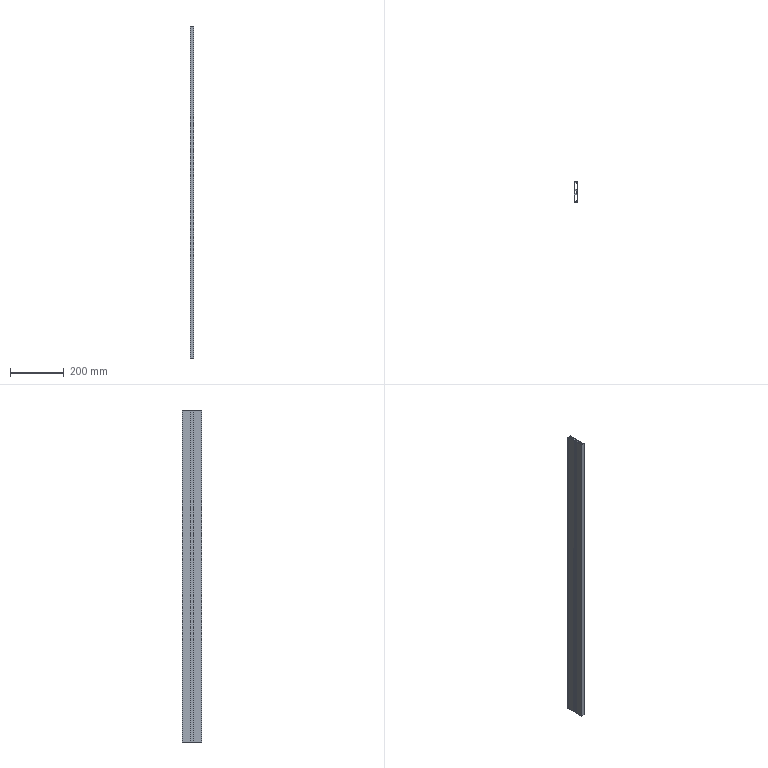Part | 1 solid | 22 faces | box 12 x 73 x 1240 mm | volume 451360 mm3 | plane 22
STEP:
#1=CARTESIAN_POINT('',(-12.,36.5,620.));
#2=VERTEX_POINT('',#1);
#3=CARTESIAN_POINT('',(-12.,4.5,620.));
#4=VERTEX_POINT('',#3);
#5=CARTESIAN_POINT('',(-12.,36.5,620.));
#6=DIRECTION('',(0.,-1.,0.));
#7=VECTOR('',#6,1000.);
#8=LINE('',#5,#7);
#9=EDGE_CURVE('',#2,#4,#8,.T.);
#10=ORIENTED_EDGE('',*,*,#9,.T.);
#11=CARTESIAN_POINT('',(-10.,4.5,620.));
#12=VERTEX_POINT('',#11);
#13=CARTESIAN_POINT('',(-12.,4.5,620.));
#14=DIRECTION('',(1.,0.,0.));
#15=VECTOR('',#14,1000.);
#16=LINE('',#13,#15);
#17=EDGE_CURVE('',#4,#12,#16,.T.);
#18=ORIENTED_EDGE('',*,*,#17,.T.);
#19=CARTESIAN_POINT('',(-10.,6.5,620.));
#20=VERTEX_POINT('',#19);
#21=CARTESIAN_POINT('',(-10.,4.5,620.));
#22=DIRECTION('',(0.,1.,0.));
#23=VECTOR('',#22,1000.);
#24=LINE('',#21,#23);
#25=EDGE_CURVE('',#12,#20,#24,.T.);
#26=ORIENTED_EDGE('',*,*,#25,.T.);
#27=CARTESIAN_POINT('',(-4.,6.5,620.));
#28=VERTEX_POINT('',#27);
#29=CARTESIAN_POINT('',(-10.,6.5,620.));
#30=DIRECTION('',(1.,0.,0.));
#31=VECTOR('',#30,1000.);
#32=LINE('',#29,#31);
#33=EDGE_CURVE('',#20,#28,#32,.T.);
#34=ORIENTED_EDGE('',*,*,#33,.T.);
#35=CARTESIAN_POINT('',(-4.,-6.5,620.));
#36=VERTEX_POINT('',#35);
#37=CARTESIAN_POINT('',(-4.,6.5,620.));
#38=DIRECTION('',(0.,-1.,0.));
#39=VECTOR('',#38,1000.);
#40=LINE('',#37,#39);
#41=EDGE_CURVE('',#28,#36,#40,.T.);
#42=ORIENTED_EDGE('',*,*,#41,.T.);
#43=CARTESIAN_POINT('',(-10.,-6.5,620.));
#44=VERTEX_POINT('',#43);
#45=CARTESIAN_POINT('',(-4.,-6.5,620.));
#46=DIRECTION('',(-1.,0.,0.));
#47=VECTOR('',#46,1000.);
#48=LINE('',#45,#47);
#49=EDGE_CURVE('',#36,#44,#48,.T.);
#50=ORIENTED_EDGE('',*,*,#49,.T.);
#51=CARTESIAN_POINT('',(-10.,-4.5,620.));
#52=VERTEX_POINT('',#51);
#53=CARTESIAN_POINT('',(-10.,-6.5,620.));
#54=DIRECTION('',(0.,1.,0.));
#55=VECTOR('',#54,1000.);
#56=LINE('',#53,#55);
#57=EDGE_CURVE('',#44,#52,#56,.T.);
#58=ORIENTED_EDGE('',*,*,#57,.T.);
#59=CARTESIAN_POINT('',(-12.,-4.5,620.));
#60=VERTEX_POINT('',#59);
#61=CARTESIAN_POINT('',(-10.,-4.5,620.));
#62=DIRECTION('',(-1.,0.,0.));
#63=VECTOR('',#62,1000.);
#64=LINE('',#61,#63);
#65=EDGE_CURVE('',#52,#60,#64,.T.);
#66=ORIENTED_EDGE('',*,*,#65,.T.);
#67=CARTESIAN_POINT('',(-12.,-36.5,620.));
#68=VERTEX_POINT('',#67);
#69=CARTESIAN_POINT('',(-12.,-4.5,620.));
#70=DIRECTION('',(0.,-1.,0.));
#71=VECTOR('',#70,1000.);
#72=LINE('',#69,#71);
#73=EDGE_CURVE('',#60,#68,#72,.T.);
#74=ORIENTED_EDGE('',*,*,#73,.T.);
#75=CARTESIAN_POINT('',(0.,-36.5,620.));
#76=VERTEX_POINT('',#75);
#77=CARTESIAN_POINT('',(-12.,-36.5,620.));
#78=DIRECTION('',(1.,0.,0.));
#79=VECTOR('',#78,1000.);
#80=LINE('',#77,#79);
#81=EDGE_CURVE('',#68,#76,#80,.T.);
#82=ORIENTED_EDGE('',*,*,#81,.T.);
#83=CARTESIAN_POINT('',(0.,36.5,620.));
#84=VERTEX_POINT('',#83);
#85=CARTESIAN_POINT('',(0.,-36.5,620.));
#86=DIRECTION('',(0.,1.,0.));
#87=VECTOR('',#86,1000.);
#88=LINE('',#85,#87);
#89=EDGE_CURVE('',#76,#84,#88,.T.);
#90=ORIENTED_EDGE('',*,*,#89,.T.);
#91=CARTESIAN_POINT('',(0.,36.5,620.));
#92=DIRECTION('',(-1.,0.,0.));
#93=VECTOR('',#92,1000.);
#94=LINE('',#91,#93);
#95=EDGE_CURVE('',#84,#2,#94,.T.);
#96=ORIENTED_EDGE('',*,*,#95,.T.);
#97=EDGE_LOOP('',(#10,#18,#26,#34,#42,#50,#58,#66,#74,#82,#90,#96));
#98=FACE_OUTER_BOUND('',#97,.T.);
#99=CARTESIAN_POINT('',(-10.,-34.5,620.));
#100=VERTEX_POINT('',#99);
#101=CARTESIAN_POINT('',(-2.,-34.5,620.));
#102=VERTEX_POINT('',#101);
#103=CARTESIAN_POINT('',(-2.,-34.5,620.));
#104=DIRECTION('',(1.,0.,0.));
#105=VECTOR('',#104,1000.);
#106=LINE('',#103,#105);
#107=EDGE_CURVE('',#100,#102,#106,.T.);
#108=ORIENTED_EDGE('',*,*,#107,.F.);
#109=CARTESIAN_POINT('',(-10.,-8.5,620.));
#110=VERTEX_POINT('',#109);
#111=CARTESIAN_POINT('',(-10.,-34.5,620.));
#112=DIRECTION('',(0.,-1.,0.));
#113=VECTOR('',#112,1000.);
#114=LINE('',#111,#113);
#115=EDGE_CURVE('',#110,#100,#114,.T.);
#116=ORIENTED_EDGE('',*,*,#115,.F.);
#117=CARTESIAN_POINT('',(-2.,-8.5,620.));
#118=VERTEX_POINT('',#117);
#119=CARTESIAN_POINT('',(-10.,-8.5,620.));
#120=DIRECTION('',(-1.,0.,0.));
#121=VECTOR('',#120,1000.);
#122=LINE('',#119,#121);
#123=EDGE_CURVE('',#118,#110,#122,.T.);
#124=ORIENTED_EDGE('',*,*,#123,.F.);
#125=CARTESIAN_POINT('',(-2.,-8.5,620.));
#126=DIRECTION('',(0.,1.,0.));
#127=VECTOR('',#126,1000.);
#128=LINE('',#125,#127);
#129=EDGE_CURVE('',#102,#118,#128,.T.);
#130=ORIENTED_EDGE('',*,*,#129,.F.);
#131=EDGE_LOOP('',(#108,#116,#124,#130));
#132=FACE_BOUND('',#131,.T.);
#133=CARTESIAN_POINT('',(-10.,34.5,620.));
#134=VERTEX_POINT('',#133);
#135=CARTESIAN_POINT('',(-10.,8.5,620.));
#136=VERTEX_POINT('',#135);
#137=CARTESIAN_POINT('',(-10.,8.5,620.));
#138=DIRECTION('',(0.,-1.,0.));
#139=VECTOR('',#138,1000.);
#140=LINE('',#137,#139);
#141=EDGE_CURVE('',#134,#136,#140,.T.);
#142=ORIENTED_EDGE('',*,*,#141,.F.);
#143=CARTESIAN_POINT('',(-2.,34.5,620.));
#144=VERTEX_POINT('',#143);
#145=CARTESIAN_POINT('',(-10.,34.5,620.));
#146=DIRECTION('',(-1.,0.,0.));
#147=VECTOR('',#146,1000.);
#148=LINE('',#145,#147);
#149=EDGE_CURVE('',#144,#134,#148,.T.);
#150=ORIENTED_EDGE('',*,*,#149,.F.);
#151=CARTESIAN_POINT('',(-2.,8.5,620.));
#152=VERTEX_POINT('',#151);
#153=CARTESIAN_POINT('',(-2.,34.5,620.));
#154=DIRECTION('',(0.,1.,0.));
#155=VECTOR('',#154,1000.);
#156=LINE('',#153,#155);
#157=EDGE_CURVE('',#152,#144,#156,.T.);
#158=ORIENTED_EDGE('',*,*,#157,.F.);
#159=CARTESIAN_POINT('',(-2.,8.5,620.));
#160=DIRECTION('',(1.,0.,0.));
#161=VECTOR('',#160,1000.);
#162=LINE('',#159,#161);
#163=EDGE_CURVE('',#136,#152,#162,.T.);
#164=ORIENTED_EDGE('',*,*,#163,.F.);
#165=EDGE_LOOP('',(#142,#150,#158,#164));
#166=FACE_BOUND('',#165,.T.);
#167=CARTESIAN_POINT('',(0.,0.,620.));
#168=DIRECTION('',(0.,0.,1.));
#169=DIRECTION('',(1.,0.,0.));
#170=AXIS2_PLACEMENT_3D('',#167,#168,#169);
#171=PLANE('',#170);
#172=ADVANCED_FACE('',(#98,#132,#166),#171,.T.);
#173=CARTESIAN_POINT('',(-10.,-8.5,-620.));
#174=VERTEX_POINT('',#173);
#175=CARTESIAN_POINT('',(-10.,-34.5,-620.));
#176=VERTEX_POINT('',#175);
#177=CARTESIAN_POINT('',(-10.,-34.5,-620.));
#178=DIRECTION('',(0.,-1.,0.));
#179=VECTOR('',#178,1000.);
#180=LINE('',#177,#179);
#181=EDGE_CURVE('',#174,#176,#180,.T.);
#182=ORIENTED_EDGE('',*,*,#181,.T.);
#183=CARTESIAN_POINT('',(-2.,-34.5,-620.));
#184=VERTEX_POINT('',#183);
#185=CARTESIAN_POINT('',(-2.,-34.5,-620.));
#186=DIRECTION('',(1.,0.,0.));
#187=VECTOR('',#186,1000.);
#188=LINE('',#185,#187);
#189=EDGE_CURVE('',#176,#184,#188,.T.);
#190=ORIENTED_EDGE('',*,*,#189,.T.);
#191=CARTESIAN_POINT('',(-2.,-8.5,-620.));
#192=VERTEX_POINT('',#191);
#193=CARTESIAN_POINT('',(-2.,-8.5,-620.));
#194=DIRECTION('',(0.,1.,0.));
#195=VECTOR('',#194,1000.);
#196=LINE('',#193,#195);
#197=EDGE_CURVE('',#184,#192,#196,.T.);
#198=ORIENTED_EDGE('',*,*,#197,.T.);
#199=CARTESIAN_POINT('',(-10.,-8.5,-620.));
#200=DIRECTION('',(-1.,0.,0.));
#201=VECTOR('',#200,1000.);
#202=LINE('',#199,#201);
#203=EDGE_CURVE('',#192,#174,#202,.T.);
#204=ORIENTED_EDGE('',*,*,#203,.T.);
#205=EDGE_LOOP('',(#182,#190,#198,#204));
#206=FACE_BOUND('',#205,.T.);
#207=CARTESIAN_POINT('',(-12.,36.5,-620.));
#208=VERTEX_POINT('',#207);
#209=CARTESIAN_POINT('',(-12.,4.5,-620.));
#210=VERTEX_POINT('',#209);
#211=CARTESIAN_POINT('',(-12.,36.5,-620.));
#212=DIRECTION('',(0.,-1.,0.));
#213=VECTOR('',#212,1000.);
#214=LINE('',#211,#213);
#215=EDGE_CURVE('',#208,#210,#214,.T.);
#216=ORIENTED_EDGE('',*,*,#215,.F.);
#217=CARTESIAN_POINT('',(0.,36.5,-620.));
#218=VERTEX_POINT('',#217);
#219=CARTESIAN_POINT('',(0.,36.5,-620.));
#220=DIRECTION('',(-1.,0.,0.));
#221=VECTOR('',#220,1000.);
#222=LINE('',#219,#221);
#223=EDGE_CURVE('',#218,#208,#222,.T.);
#224=ORIENTED_EDGE('',*,*,#223,.F.);
#225=CARTESIAN_POINT('',(0.,-36.5,-620.));
#226=VERTEX_POINT('',#225);
#227=CARTESIAN_POINT('',(0.,-36.5,-620.));
#228=DIRECTION('',(0.,1.,0.));
#229=VECTOR('',#228,1000.);
#230=LINE('',#227,#229);
#231=EDGE_CURVE('',#226,#218,#230,.T.);
#232=ORIENTED_EDGE('',*,*,#231,.F.);
#233=CARTESIAN_POINT('',(-12.,-36.5,-620.));
#234=VERTEX_POINT('',#233);
#235=CARTESIAN_POINT('',(-12.,-36.5,-620.));
#236=DIRECTION('',(1.,0.,0.));
#237=VECTOR('',#236,1000.);
#238=LINE('',#235,#237);
#239=EDGE_CURVE('',#234,#226,#238,.T.);
#240=ORIENTED_EDGE('',*,*,#239,.F.);
#241=CARTESIAN_POINT('',(-12.,-4.5,-620.));
#242=VERTEX_POINT('',#241);
#243=CARTESIAN_POINT('',(-12.,-4.5,-620.));
#244=DIRECTION('',(0.,-1.,0.));
#245=VECTOR('',#244,1000.);
#246=LINE('',#243,#245);
#247=EDGE_CURVE('',#242,#234,#246,.T.);
#248=ORIENTED_EDGE('',*,*,#247,.F.);
#249=CARTESIAN_POINT('',(-10.,-4.5,-620.));
#250=VERTEX_POINT('',#249);
#251=CARTESIAN_POINT('',(-10.,-4.5,-620.));
#252=DIRECTION('',(-1.,0.,0.));
#253=VECTOR('',#252,1000.);
#254=LINE('',#251,#253);
#255=EDGE_CURVE('',#250,#242,#254,.T.);
#256=ORIENTED_EDGE('',*,*,#255,.F.);
#257=CARTESIAN_POINT('',(-10.,-6.5,-620.));
#258=VERTEX_POINT('',#257);
#259=CARTESIAN_POINT('',(-10.,-6.5,-620.));
#260=DIRECTION('',(0.,1.,0.));
#261=VECTOR('',#260,1000.);
#262=LINE('',#259,#261);
#263=EDGE_CURVE('',#258,#250,#262,.T.);
#264=ORIENTED_EDGE('',*,*,#263,.F.);
#265=CARTESIAN_POINT('',(-4.,-6.5,-620.));
#266=VERTEX_POINT('',#265);
#267=CARTESIAN_POINT('',(-4.,-6.5,-620.));
#268=DIRECTION('',(-1.,0.,0.));
#269=VECTOR('',#268,1000.);
#270=LINE('',#267,#269);
#271=EDGE_CURVE('',#266,#258,#270,.T.);
#272=ORIENTED_EDGE('',*,*,#271,.F.);
#273=CARTESIAN_POINT('',(-4.,6.5,-620.));
#274=VERTEX_POINT('',#273);
#275=CARTESIAN_POINT('',(-4.,6.5,-620.));
#276=DIRECTION('',(0.,-1.,0.));
#277=VECTOR('',#276,1000.);
#278=LINE('',#275,#277);
#279=EDGE_CURVE('',#274,#266,#278,.T.);
#280=ORIENTED_EDGE('',*,*,#279,.F.);
#281=CARTESIAN_POINT('',(-10.,6.5,-620.));
#282=VERTEX_POINT('',#281);
#283=CARTESIAN_POINT('',(-10.,6.5,-620.));
#284=DIRECTION('',(1.,0.,0.));
#285=VECTOR('',#284,1000.);
#286=LINE('',#283,#285);
#287=EDGE_CURVE('',#282,#274,#286,.T.);
#288=ORIENTED_EDGE('',*,*,#287,.F.);
#289=CARTESIAN_POINT('',(-10.,4.5,-620.));
#290=VERTEX_POINT('',#289);
#291=CARTESIAN_POINT('',(-10.,4.5,-620.));
#292=DIRECTION('',(0.,1.,0.));
#293=VECTOR('',#292,1000.);
#294=LINE('',#291,#293);
#295=EDGE_CURVE('',#290,#282,#294,.T.);
#296=ORIENTED_EDGE('',*,*,#295,.F.);
#297=CARTESIAN_POINT('',(-12.,4.5,-620.));
#298=DIRECTION('',(1.,0.,0.));
#299=VECTOR('',#298,1000.);
#300=LINE('',#297,#299);
#301=EDGE_CURVE('',#210,#290,#300,.T.);
#302=ORIENTED_EDGE('',*,*,#301,.F.);
#303=EDGE_LOOP('',(#216,#224,#232,#240,#248,#256,#264,#272,#280,#288,#296,#302));
#304=FACE_OUTER_BOUND('',#303,.T.);
#305=CARTESIAN_POINT('',(-2.,34.5,-620.));
#306=VERTEX_POINT('',#305);
#307=CARTESIAN_POINT('',(-10.,34.5,-620.));
#308=VERTEX_POINT('',#307);
#309=CARTESIAN_POINT('',(-10.,34.5,-620.));
#310=DIRECTION('',(-1.,0.,0.));
#311=VECTOR('',#310,1000.);
#312=LINE('',#309,#311);
#313=EDGE_CURVE('',#306,#308,#312,.T.);
#314=ORIENTED_EDGE('',*,*,#313,.T.);
#315=CARTESIAN_POINT('',(-10.,8.5,-620.));
#316=VERTEX_POINT('',#315);
#317=CARTESIAN_POINT('',(-10.,8.5,-620.));
#318=DIRECTION('',(0.,-1.,0.));
#319=VECTOR('',#318,1000.);
#320=LINE('',#317,#319);
#321=EDGE_CURVE('',#308,#316,#320,.T.);
#322=ORIENTED_EDGE('',*,*,#321,.T.);
#323=CARTESIAN_POINT('',(-2.,8.5,-620.));
#324=VERTEX_POINT('',#323);
#325=CARTESIAN_POINT('',(-2.,8.5,-620.));
#326=DIRECTION('',(1.,0.,0.));
#327=VECTOR('',#326,1000.);
#328=LINE('',#325,#327);
#329=EDGE_CURVE('',#316,#324,#328,.T.);
#330=ORIENTED_EDGE('',*,*,#329,.T.);
#331=CARTESIAN_POINT('',(-2.,34.5,-620.));
#332=DIRECTION('',(0.,1.,0.));
#333=VECTOR('',#332,1000.);
#334=LINE('',#331,#333);
#335=EDGE_CURVE('',#324,#306,#334,.T.);
#336=ORIENTED_EDGE('',*,*,#335,.T.);
#337=EDGE_LOOP('',(#314,#322,#330,#336));
#338=FACE_BOUND('',#337,.T.);
#339=CARTESIAN_POINT('',(0.,0.,-620.));
#340=DIRECTION('',(0.,0.,1.));
#341=DIRECTION('',(1.,0.,0.));
#342=AXIS2_PLACEMENT_3D('',#339,#340,#341);
#343=PLANE('',#342);
#344=ADVANCED_FACE('',(#206,#304,#338),#343,.F.);
#345=ORIENTED_EDGE('',*,*,#215,.T.);
#346=CARTESIAN_POINT('',(-12.,4.5,620.));
#347=DIRECTION('',(0.,0.,-1.));
#348=VECTOR('',#347,1000.);
#349=LINE('',#346,#348);
#350=EDGE_CURVE('',#4,#210,#349,.T.);
#351=ORIENTED_EDGE('',*,*,#350,.F.);
#352=ORIENTED_EDGE('',*,*,#9,.F.);
#353=CARTESIAN_POINT('',(-12.,36.5,620.));
#354=DIRECTION('',(0.,0.,-1.));
#355=VECTOR('',#354,1000.);
#356=LINE('',#353,#355);
#357=EDGE_CURVE('',#2,#208,#356,.T.);
#358=ORIENTED_EDGE('',*,*,#357,.T.);
#359=EDGE_LOOP('',(#345,#351,#352,#358));
#360=FACE_OUTER_BOUND('',#359,.T.);
#361=CARTESIAN_POINT('',(-12.,36.5,620.));
#362=DIRECTION('',(1.,0.,0.));
#363=DIRECTION('',(0.,0.,-1.));
#364=AXIS2_PLACEMENT_3D('',#361,#362,#363);
#365=PLANE('',#364);
#366=ADVANCED_FACE('',(#360),#365,.F.);
#367=ORIENTED_EDGE('',*,*,#301,.T.);
#368=CARTESIAN_POINT('',(-10.,4.5,620.));
#369=DIRECTION('',(0.,0.,-1.));
#370=VECTOR('',#369,1000.);
#371=LINE('',#368,#370);
#372=EDGE_CURVE('',#12,#290,#371,.T.);
#373=ORIENTED_EDGE('',*,*,#372,.F.);
#374=ORIENTED_EDGE('',*,*,#17,.F.);
#375=ORIENTED_EDGE('',*,*,#350,.T.);
#376=EDGE_LOOP('',(#367,#373,#374,#375));
#377=FACE_OUTER_BOUND('',#376,.T.);
#378=CARTESIAN_POINT('',(-12.,4.5,620.));
#379=DIRECTION('',(0.,1.,0.));
#380=DIRECTION('',(0.,0.,1.));
#381=AXIS2_PLACEMENT_3D('',#378,#379,#380);
#382=PLANE('',#381);
#383=ADVANCED_FACE('',(#377),#382,.F.);
#384=ORIENTED_EDGE('',*,*,#295,.T.);
#385=CARTESIAN_POINT('',(-10.,6.5,620.));
#386=DIRECTION('',(0.,0.,-1.));
#387=VECTOR('',#386,1000.);
#388=LINE('',#385,#387);
#389=EDGE_CURVE('',#20,#282,#388,.T.);
#390=ORIENTED_EDGE('',*,*,#389,.F.);
#391=ORIENTED_EDGE('',*,*,#25,.F.);
#392=ORIENTED_EDGE('',*,*,#372,.T.);
#393=EDGE_LOOP('',(#384,#390,#391,#392));
#394=FACE_OUTER_BOUND('',#393,.T.);
#395=CARTESIAN_POINT('',(-10.,4.5,620.));
#396=DIRECTION('',(-1.,0.,0.));
#397=DIRECTION('',(0.,0.,1.));
#398=AXIS2_PLACEMENT_3D('',#395,#396,#397);
#399=PLANE('',#398);
#400=ADVANCED_FACE('',(#394),#399,.F.);
#401=ORIENTED_EDGE('',*,*,#287,.T.);
#402=CARTESIAN_POINT('',(-4.,6.5,620.));
#403=DIRECTION('',(0.,0.,-1.));
#404=VECTOR('',#403,1000.);
#405=LINE('',#402,#404);
#406=EDGE_CURVE('',#28,#274,#405,.T.);
#407=ORIENTED_EDGE('',*,*,#406,.F.);
#408=ORIENTED_EDGE('',*,*,#33,.F.);
#409=ORIENTED_EDGE('',*,*,#389,.T.);
#410=EDGE_LOOP('',(#401,#407,#408,#409));
#411=FACE_OUTER_BOUND('',#410,.T.);
#412=CARTESIAN_POINT('',(-10.,6.5,620.));
#413=DIRECTION('',(0.,1.,0.));
#414=DIRECTION('',(0.,0.,1.));
#415=AXIS2_PLACEMENT_3D('',#412,#413,#414);
#416=PLANE('',#415);
#417=ADVANCED_FACE('',(#411),#416,.F.);
#418=ORIENTED_EDGE('',*,*,#279,.T.);
#419=CARTESIAN_POINT('',(-4.,-6.5,620.));
#420=DIRECTION('',(0.,0.,-1.));
#421=VECTOR('',#420,1000.);
#422=LINE('',#419,#421);
#423=EDGE_CURVE('',#36,#266,#422,.T.);
#424=ORIENTED_EDGE('',*,*,#423,.F.);
#425=ORIENTED_EDGE('',*,*,#41,.F.);
#426=ORIENTED_EDGE('',*,*,#406,.T.);
#427=EDGE_LOOP('',(#418,#424,#425,#426));
#428=FACE_OUTER_BOUND('',#427,.T.);
#429=CARTESIAN_POINT('',(-4.,6.5,620.));
#430=DIRECTION('',(1.,0.,0.));
#431=DIRECTION('',(0.,0.,-1.));
#432=AXIS2_PLACEMENT_3D('',#429,#430,#431);
#433=PLANE('',#432);
#434=ADVANCED_FACE('',(#428),#433,.F.);
#435=ORIENTED_EDGE('',*,*,#271,.T.);
#436=CARTESIAN_POINT('',(-10.,-6.5,620.));
#437=DIRECTION('',(0.,0.,-1.));
#438=VECTOR('',#437,1000.);
#439=LINE('',#436,#438);
#440=EDGE_CURVE('',#44,#258,#439,.T.);
#441=ORIENTED_EDGE('',*,*,#440,.F.);
#442=ORIENTED_EDGE('',*,*,#49,.F.);
#443=ORIENTED_EDGE('',*,*,#423,.T.);
#444=EDGE_LOOP('',(#435,#441,#442,#443));
#445=FACE_OUTER_BOUND('',#444,.T.);
#446=CARTESIAN_POINT('',(-4.,-6.5,620.));
#447=DIRECTION('',(0.,-1.,0.));
#448=DIRECTION('',(0.,0.,-1.));
#449=AXIS2_PLACEMENT_3D('',#446,#447,#448);
#450=PLANE('',#449);
#451=ADVANCED_FACE('',(#445),#450,.F.);
#452=ORIENTED_EDGE('',*,*,#263,.T.);
#453=CARTESIAN_POINT('',(-10.,-4.5,620.));
#454=DIRECTION('',(0.,0.,-1.));
#455=VECTOR('',#454,1000.);
#456=LINE('',#453,#455);
#457=EDGE_CURVE('',#52,#250,#456,.T.);
#458=ORIENTED_EDGE('',*,*,#457,.F.);
#459=ORIENTED_EDGE('',*,*,#57,.F.);
#460=ORIENTED_EDGE('',*,*,#440,.T.);
#461=EDGE_LOOP('',(#452,#458,#459,#460));
#462=FACE_OUTER_BOUND('',#461,.T.);
#463=CARTESIAN_POINT('',(-10.,-6.5,620.));
#464=DIRECTION('',(-1.,0.,0.));
#465=DIRECTION('',(0.,0.,1.));
#466=AXIS2_PLACEMENT_3D('',#463,#464,#465);
#467=PLANE('',#466);
#468=ADVANCED_FACE('',(#462),#467,.F.);
#469=ORIENTED_EDGE('',*,*,#255,.T.);
#470=CARTESIAN_POINT('',(-12.,-4.5,620.));
#471=DIRECTION('',(0.,0.,-1.));
#472=VECTOR('',#471,1000.);
#473=LINE('',#470,#472);
#474=EDGE_CURVE('',#60,#242,#473,.T.);
#475=ORIENTED_EDGE('',*,*,#474,.F.);
#476=ORIENTED_EDGE('',*,*,#65,.F.);
#477=ORIENTED_EDGE('',*,*,#457,.T.);
#478=EDGE_LOOP('',(#469,#475,#476,#477));
#479=FACE_OUTER_BOUND('',#478,.T.);
#480=CARTESIAN_POINT('',(-10.,-4.5,620.));
#481=DIRECTION('',(0.,-1.,0.));
#482=DIRECTION('',(0.,0.,-1.));
#483=AXIS2_PLACEMENT_3D('',#480,#481,#482);
#484=PLANE('',#483);
#485=ADVANCED_FACE('',(#479),#484,.F.);
#486=ORIENTED_EDGE('',*,*,#247,.T.);
#487=CARTESIAN_POINT('',(-12.,-36.5,620.));
#488=DIRECTION('',(0.,0.,-1.));
#489=VECTOR('',#488,1000.);
#490=LINE('',#487,#489);
#491=EDGE_CURVE('',#68,#234,#490,.T.);
#492=ORIENTED_EDGE('',*,*,#491,.F.);
#493=ORIENTED_EDGE('',*,*,#73,.F.);
#494=ORIENTED_EDGE('',*,*,#474,.T.);
#495=EDGE_LOOP('',(#486,#492,#493,#494));
#496=FACE_OUTER_BOUND('',#495,.T.);
#497=CARTESIAN_POINT('',(-12.,-4.5,620.));
#498=DIRECTION('',(1.,0.,0.));
#499=DIRECTION('',(0.,0.,-1.));
#500=AXIS2_PLACEMENT_3D('',#497,#498,#499);
#501=PLANE('',#500);
#502=ADVANCED_FACE('',(#496),#501,.F.);
#503=ORIENTED_EDGE('',*,*,#239,.T.);
#504=CARTESIAN_POINT('',(0.,-36.5,620.));
#505=DIRECTION('',(0.,0.,-1.));
#506=VECTOR('',#505,1000.);
#507=LINE('',#504,#506);
#508=EDGE_CURVE('',#76,#226,#507,.T.);
#509=ORIENTED_EDGE('',*,*,#508,.F.);
#510=ORIENTED_EDGE('',*,*,#81,.F.);
#511=ORIENTED_EDGE('',*,*,#491,.T.);
#512=EDGE_LOOP('',(#503,#509,#510,#511));
#513=FACE_OUTER_BOUND('',#512,.T.);
#514=CARTESIAN_POINT('',(-12.,-36.5,620.));
#515=DIRECTION('',(0.,1.,0.));
#516=DIRECTION('',(0.,0.,1.));
#517=AXIS2_PLACEMENT_3D('',#514,#515,#516);
#518=PLANE('',#517);
#519=ADVANCED_FACE('',(#513),#518,.F.);
#520=ORIENTED_EDGE('',*,*,#231,.T.);
#521=CARTESIAN_POINT('',(0.,36.5,620.));
#522=DIRECTION('',(0.,0.,-1.));
#523=VECTOR('',#522,1000.);
#524=LINE('',#521,#523);
#525=EDGE_CURVE('',#84,#218,#524,.T.);
#526=ORIENTED_EDGE('',*,*,#525,.F.);
#527=ORIENTED_EDGE('',*,*,#89,.F.);
#528=ORIENTED_EDGE('',*,*,#508,.T.);
#529=EDGE_LOOP('',(#520,#526,#527,#528));
#530=FACE_OUTER_BOUND('',#529,.T.);
#531=CARTESIAN_POINT('',(0.,-36.5,620.));
#532=DIRECTION('',(-1.,0.,0.));
#533=DIRECTION('',(0.,0.,1.));
#534=AXIS2_PLACEMENT_3D('',#531,#532,#533);
#535=PLANE('',#534);
#536=ADVANCED_FACE('',(#530),#535,.F.);
#537=ORIENTED_EDGE('',*,*,#223,.T.);
#538=ORIENTED_EDGE('',*,*,#357,.F.);
#539=ORIENTED_EDGE('',*,*,#95,.F.);
#540=ORIENTED_EDGE('',*,*,#525,.T.);
#541=EDGE_LOOP('',(#537,#538,#539,#540));
#542=FACE_OUTER_BOUND('',#541,.T.);
#543=CARTESIAN_POINT('',(0.,36.5,620.));
#544=DIRECTION('',(0.,-1.,0.));
#545=DIRECTION('',(0.,0.,-1.));
#546=AXIS2_PLACEMENT_3D('',#543,#544,#545);
#547=PLANE('',#546);
#548=ADVANCED_FACE('',(#542),#547,.F.);
#549=ORIENTED_EDGE('',*,*,#181,.F.);
#550=CARTESIAN_POINT('',(-10.,-8.5,620.));
#551=DIRECTION('',(0.,0.,-1.));
#552=VECTOR('',#551,1000.);
#553=LINE('',#550,#552);
#554=EDGE_CURVE('',#110,#174,#553,.T.);
#555=ORIENTED_EDGE('',*,*,#554,.F.);
#556=ORIENTED_EDGE('',*,*,#115,.T.);
#557=CARTESIAN_POINT('',(-10.,-34.5,620.));
#558=DIRECTION('',(0.,0.,-1.));
#559=VECTOR('',#558,1000.);
#560=LINE('',#557,#559);
#561=EDGE_CURVE('',#100,#176,#560,.T.);
#562=ORIENTED_EDGE('',*,*,#561,.T.);
#563=EDGE_LOOP('',(#549,#555,#556,#562));
#564=FACE_OUTER_BOUND('',#563,.T.);
#565=CARTESIAN_POINT('',(-10.,-34.5,620.));
#566=DIRECTION('',(1.,0.,0.));
#567=DIRECTION('',(0.,0.,-1.));
#568=AXIS2_PLACEMENT_3D('',#565,#566,#567);
#569=PLANE('',#568);
#570=ADVANCED_FACE('',(#564),#569,.T.);
#571=ORIENTED_EDGE('',*,*,#189,.F.);
#572=ORIENTED_EDGE('',*,*,#561,.F.);
#573=ORIENTED_EDGE('',*,*,#107,.T.);
#574=CARTESIAN_POINT('',(-2.,-34.5,620.));
#575=DIRECTION('',(0.,0.,-1.));
#576=VECTOR('',#575,1000.);
#577=LINE('',#574,#576);
#578=EDGE_CURVE('',#102,#184,#577,.T.);
#579=ORIENTED_EDGE('',*,*,#578,.T.);
#580=EDGE_LOOP('',(#571,#572,#573,#579));
#581=FACE_OUTER_BOUND('',#580,.T.);
#582=CARTESIAN_POINT('',(-2.,-34.5,620.));
#583=DIRECTION('',(0.,1.,0.));
#584=DIRECTION('',(0.,0.,1.));
#585=AXIS2_PLACEMENT_3D('',#582,#583,#584);
#586=PLANE('',#585);
#587=ADVANCED_FACE('',(#581),#586,.T.);
#588=ORIENTED_EDGE('',*,*,#197,.F.);
#589=ORIENTED_EDGE('',*,*,#578,.F.);
#590=ORIENTED_EDGE('',*,*,#129,.T.);
#591=CARTESIAN_POINT('',(-2.,-8.5,620.));
#592=DIRECTION('',(0.,0.,-1.));
#593=VECTOR('',#592,1000.);
#594=LINE('',#591,#593);
#595=EDGE_CURVE('',#118,#192,#594,.T.);
#596=ORIENTED_EDGE('',*,*,#595,.T.);
#597=EDGE_LOOP('',(#588,#589,#590,#596));
#598=FACE_OUTER_BOUND('',#597,.T.);
#599=CARTESIAN_POINT('',(-2.,-8.5,620.));
#600=DIRECTION('',(-1.,0.,0.));
#601=DIRECTION('',(0.,0.,1.));
#602=AXIS2_PLACEMENT_3D('',#599,#600,#601);
#603=PLANE('',#602);
#604=ADVANCED_FACE('',(#598),#603,.T.);
#605=ORIENTED_EDGE('',*,*,#203,.F.);
#606=ORIENTED_EDGE('',*,*,#595,.F.);
#607=ORIENTED_EDGE('',*,*,#123,.T.);
#608=ORIENTED_EDGE('',*,*,#554,.T.);
#609=EDGE_LOOP('',(#605,#606,#607,#608));
#610=FACE_OUTER_BOUND('',#609,.T.);
#611=CARTESIAN_POINT('',(-10.,-8.5,620.));
#612=DIRECTION('',(0.,-1.,0.));
#613=DIRECTION('',(0.,0.,-1.));
#614=AXIS2_PLACEMENT_3D('',#611,#612,#613);
#615=PLANE('',#614);
#616=ADVANCED_FACE('',(#610),#615,.T.);
#617=ORIENTED_EDGE('',*,*,#313,.F.);
#618=CARTESIAN_POINT('',(-2.,34.5,620.));
#619=DIRECTION('',(0.,0.,-1.));
#620=VECTOR('',#619,1000.);
#621=LINE('',#618,#620);
#622=EDGE_CURVE('',#144,#306,#621,.T.);
#623=ORIENTED_EDGE('',*,*,#622,.F.);
#624=ORIENTED_EDGE('',*,*,#149,.T.);
#625=CARTESIAN_POINT('',(-10.,34.5,620.));
#626=DIRECTION('',(0.,0.,-1.));
#627=VECTOR('',#626,1000.);
#628=LINE('',#625,#627);
#629=EDGE_CURVE('',#134,#308,#628,.T.);
#630=ORIENTED_EDGE('',*,*,#629,.T.);
#631=EDGE_LOOP('',(#617,#623,#624,#630));
#632=FACE_OUTER_BOUND('',#631,.T.);
#633=CARTESIAN_POINT('',(-10.,34.5,620.));
#634=DIRECTION('',(0.,-1.,0.));
#635=DIRECTION('',(0.,0.,-1.));
#636=AXIS2_PLACEMENT_3D('',#633,#634,#635);
#637=PLANE('',#636);
#638=ADVANCED_FACE('',(#632),#637,.T.);
#639=ORIENTED_EDGE('',*,*,#321,.F.);
#640=ORIENTED_EDGE('',*,*,#629,.F.);
#641=ORIENTED_EDGE('',*,*,#141,.T.);
#642=CARTESIAN_POINT('',(-10.,8.5,620.));
#643=DIRECTION('',(0.,0.,-1.));
#644=VECTOR('',#643,1000.);
#645=LINE('',#642,#644);
#646=EDGE_CURVE('',#136,#316,#645,.T.);
#647=ORIENTED_EDGE('',*,*,#646,.T.);
#648=EDGE_LOOP('',(#639,#640,#641,#647));
#649=FACE_OUTER_BOUND('',#648,.T.);
#650=CARTESIAN_POINT('',(-10.,8.5,620.));
#651=DIRECTION('',(1.,0.,0.));
#652=DIRECTION('',(0.,0.,-1.));
#653=AXIS2_PLACEMENT_3D('',#650,#651,#652);
#654=PLANE('',#653);
#655=ADVANCED_FACE('',(#649),#654,.T.);
#656=ORIENTED_EDGE('',*,*,#329,.F.);
#657=ORIENTED_EDGE('',*,*,#646,.F.);
#658=ORIENTED_EDGE('',*,*,#163,.T.);
#659=CARTESIAN_POINT('',(-2.,8.5,620.));
#660=DIRECTION('',(0.,0.,-1.));
#661=VECTOR('',#660,1000.);
#662=LINE('',#659,#661);
#663=EDGE_CURVE('',#152,#324,#662,.T.);
#664=ORIENTED_EDGE('',*,*,#663,.T.);
#665=EDGE_LOOP('',(#656,#657,#658,#664));
#666=FACE_OUTER_BOUND('',#665,.T.);
#667=CARTESIAN_POINT('',(-2.,8.5,620.));
#668=DIRECTION('',(0.,1.,0.));
#669=DIRECTION('',(0.,0.,1.));
#670=AXIS2_PLACEMENT_3D('',#667,#668,#669);
#671=PLANE('',#670);
#672=ADVANCED_FACE('',(#666),#671,.T.);
#673=ORIENTED_EDGE('',*,*,#335,.F.);
#674=ORIENTED_EDGE('',*,*,#663,.F.);
#675=ORIENTED_EDGE('',*,*,#157,.T.);
#676=ORIENTED_EDGE('',*,*,#622,.T.);
#677=EDGE_LOOP('',(#673,#674,#675,#676));
#678=FACE_OUTER_BOUND('',#677,.T.);
#679=CARTESIAN_POINT('',(-2.,34.5,620.));
#680=DIRECTION('',(-1.,0.,0.));
#681=DIRECTION('',(0.,0.,1.));
#682=AXIS2_PLACEMENT_3D('',#679,#680,#681);
#683=PLANE('',#682);
#684=ADVANCED_FACE('',(#678),#683,.T.);
#685=CLOSED_SHELL('',(#172,#344,#366,#383,#400,#417,#434,#451,#468,#485,#502,#519,#536,#548,#570,#587,#604,#616,#638,#655,#672,#684));
#686=MANIFOLD_SOLID_BREP('',#685);
#687=CARTESIAN_POINT('',(0.,0.,0.));
#688=DIRECTION('',(0.,0.,1.));
#689=DIRECTION('',(1.,0.,0.));
#690=AXIS2_PLACEMENT_3D('',#687,#688,#689);
#691=(LENGTH_UNIT()NAMED_UNIT(*)SI_UNIT(.MILLI.,.METRE.));
#692=UNCERTAINTY_MEASURE_WITH_UNIT(LENGTH_MEASURE(0.00001),#691,'','');
#693=(NAMED_UNIT(*)PLANE_ANGLE_UNIT()SI_UNIT($,.RADIAN.));
#694=(NAMED_UNIT(*)SI_UNIT($,.STERADIAN.)SOLID_ANGLE_UNIT());
#695=(GEOMETRIC_REPRESENTATION_CONTEXT(3)GLOBAL_UNCERTAINTY_ASSIGNED_CONTEXT((#692))GLOBAL_UNIT_ASSIGNED_CONTEXT((#691,#693,#694))REPRESENTATION_CONTEXT('',''));
#696=ADVANCED_BREP_SHAPE_REPRESENTATION('',(#686,#690),#695);